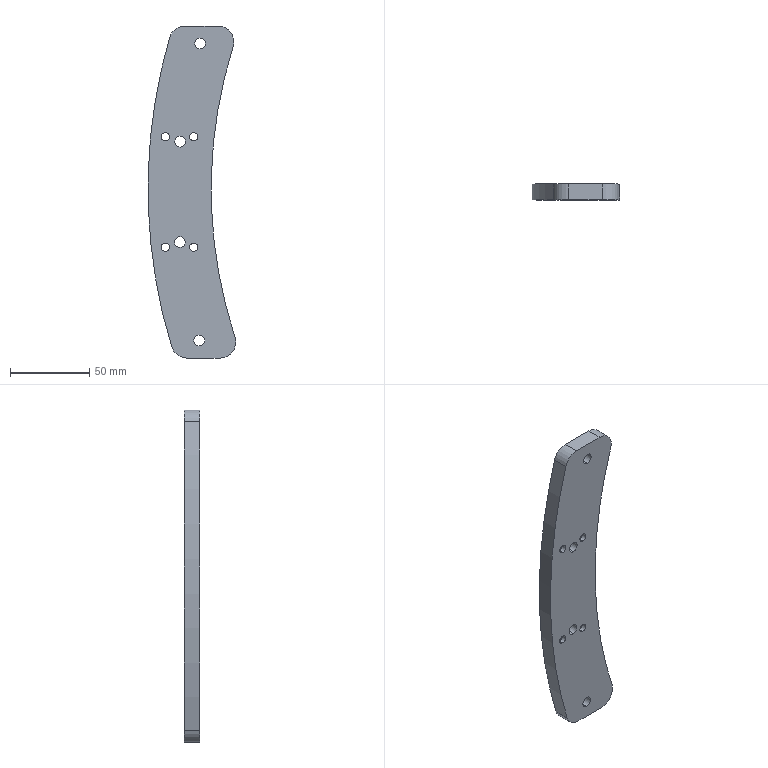Part | 1 solid | 38 faces | box 55.542 x 10 x 210 mm | volume 81183 mm3 | cylinder 30 | plane 8 | commonest cylinder face diameters 5.2 x8 6.8 x8 8.5 x8 20 x4 598 x1 682.4 x1
STEP:
#1=CARTESIAN_POINT('',(-4.991,3.,-65.75));
#2=VERTEX_POINT('',#1);
#3=CARTESIAN_POINT('',(-4.991,3.,-74.25));
#4=VERTEX_POINT('',#3);
#5=CARTESIAN_POINT('',(-4.991,3.,-70.));
#6=DIRECTION('',(0.,-1.,0.));
#7=DIRECTION('',(0.,0.,-1.));
#8=AXIS2_PLACEMENT_3D('',#5,#6,#7);
#9=CIRCLE('',#8,4.25);
#10=EDGE_CURVE('',#2,#4,#9,.T.);
#11=ORIENTED_EDGE('',*,*,#10,.T.);
#12=CARTESIAN_POINT('',(-4.991,10.,-74.25));
#13=VERTEX_POINT('',#12);
#14=CARTESIAN_POINT('',(-4.991,3.,-74.25));
#15=DIRECTION('',(0.,1.,0.));
#16=VECTOR('',#15,1000.);
#17=LINE('',#14,#16);
#18=EDGE_CURVE('',#4,#13,#17,.T.);
#19=ORIENTED_EDGE('',*,*,#18,.T.);
#20=CARTESIAN_POINT('',(-4.991,10.,-65.75));
#21=VERTEX_POINT('',#20);
#22=CARTESIAN_POINT('',(-4.991,10.,-70.));
#23=DIRECTION('',(0.,-1.,0.));
#24=DIRECTION('',(0.,0.,-1.));
#25=AXIS2_PLACEMENT_3D('',#22,#23,#24);
#26=CIRCLE('',#25,4.25);
#27=EDGE_CURVE('',#21,#13,#26,.T.);
#28=ORIENTED_EDGE('',*,*,#27,.F.);
#29=CARTESIAN_POINT('',(-4.991,3.,-65.75));
#30=DIRECTION('',(0.,1.,0.));
#31=VECTOR('',#30,1000.);
#32=LINE('',#29,#31);
#33=EDGE_CURVE('',#2,#21,#32,.T.);
#34=ORIENTED_EDGE('',*,*,#33,.F.);
#35=EDGE_LOOP('',(#11,#19,#28,#34));
#36=FACE_OUTER_BOUND('',#35,.T.);
#37=CARTESIAN_POINT('',(-4.991,3.,-70.));
#38=DIRECTION('',(0.,1.,0.));
#39=DIRECTION('',(0.,0.,1.));
#40=AXIS2_PLACEMENT_3D('',#37,#38,#39);
#41=CYLINDRICAL_SURFACE('',#40,4.25);
#42=ADVANCED_FACE('',(#36),#41,.F.);
#43=CARTESIAN_POINT('',(-4.991,3.,-135.75));
#44=VERTEX_POINT('',#43);
#45=CARTESIAN_POINT('',(-4.991,3.,-144.25));
#46=VERTEX_POINT('',#45);
#47=CARTESIAN_POINT('',(-4.991,3.,-140.));
#48=DIRECTION('',(0.,-1.,0.));
#49=DIRECTION('',(0.,0.,-1.));
#50=AXIS2_PLACEMENT_3D('',#47,#48,#49);
#51=CIRCLE('',#50,4.25);
#52=EDGE_CURVE('',#44,#46,#51,.T.);
#53=ORIENTED_EDGE('',*,*,#52,.T.);
#54=CARTESIAN_POINT('',(-4.991,10.,-144.25));
#55=VERTEX_POINT('',#54);
#56=CARTESIAN_POINT('',(-4.991,3.,-144.25));
#57=DIRECTION('',(0.,1.,0.));
#58=VECTOR('',#57,1000.);
#59=LINE('',#56,#58);
#60=EDGE_CURVE('',#46,#55,#59,.T.);
#61=ORIENTED_EDGE('',*,*,#60,.T.);
#62=CARTESIAN_POINT('',(-4.991,10.,-135.75));
#63=VERTEX_POINT('',#62);
#64=CARTESIAN_POINT('',(-4.991,10.,-140.));
#65=DIRECTION('',(0.,-1.,0.));
#66=DIRECTION('',(0.,0.,-1.));
#67=AXIS2_PLACEMENT_3D('',#64,#65,#66);
#68=CIRCLE('',#67,4.25);
#69=EDGE_CURVE('',#63,#55,#68,.T.);
#70=ORIENTED_EDGE('',*,*,#69,.F.);
#71=CARTESIAN_POINT('',(-4.991,3.,-135.75));
#72=DIRECTION('',(0.,1.,0.));
#73=VECTOR('',#72,1000.);
#74=LINE('',#71,#73);
#75=EDGE_CURVE('',#44,#63,#74,.T.);
#76=ORIENTED_EDGE('',*,*,#75,.F.);
#77=EDGE_LOOP('',(#53,#61,#70,#76));
#78=FACE_OUTER_BOUND('',#77,.T.);
#79=CARTESIAN_POINT('',(-4.991,3.,-140.));
#80=DIRECTION('',(0.,1.,0.));
#81=DIRECTION('',(0.,0.,1.));
#82=AXIS2_PLACEMENT_3D('',#79,#80,#81);
#83=CYLINDRICAL_SURFACE('',#82,4.25);
#84=ADVANCED_FACE('',(#78),#83,.F.);
#85=CARTESIAN_POINT('',(13.009,3.,-135.75));
#86=VERTEX_POINT('',#85);
#87=CARTESIAN_POINT('',(13.009,3.,-144.25));
#88=VERTEX_POINT('',#87);
#89=CARTESIAN_POINT('',(13.009,3.,-140.));
#90=DIRECTION('',(0.,-1.,0.));
#91=DIRECTION('',(0.,0.,-1.));
#92=AXIS2_PLACEMENT_3D('',#89,#90,#91);
#93=CIRCLE('',#92,4.25);
#94=EDGE_CURVE('',#86,#88,#93,.T.);
#95=ORIENTED_EDGE('',*,*,#94,.T.);
#96=CARTESIAN_POINT('',(13.009,10.,-144.25));
#97=VERTEX_POINT('',#96);
#98=CARTESIAN_POINT('',(13.009,3.,-144.25));
#99=DIRECTION('',(0.,1.,0.));
#100=VECTOR('',#99,1000.);
#101=LINE('',#98,#100);
#102=EDGE_CURVE('',#88,#97,#101,.T.);
#103=ORIENTED_EDGE('',*,*,#102,.T.);
#104=CARTESIAN_POINT('',(13.009,10.,-135.75));
#105=VERTEX_POINT('',#104);
#106=CARTESIAN_POINT('',(13.009,10.,-140.));
#107=DIRECTION('',(0.,-1.,0.));
#108=DIRECTION('',(0.,0.,-1.));
#109=AXIS2_PLACEMENT_3D('',#106,#107,#108);
#110=CIRCLE('',#109,4.25);
#111=EDGE_CURVE('',#105,#97,#110,.T.);
#112=ORIENTED_EDGE('',*,*,#111,.F.);
#113=CARTESIAN_POINT('',(13.009,3.,-135.75));
#114=DIRECTION('',(0.,1.,0.));
#115=VECTOR('',#114,1000.);
#116=LINE('',#113,#115);
#117=EDGE_CURVE('',#86,#105,#116,.T.);
#118=ORIENTED_EDGE('',*,*,#117,.F.);
#119=EDGE_LOOP('',(#95,#103,#112,#118));
#120=FACE_OUTER_BOUND('',#119,.T.);
#121=CARTESIAN_POINT('',(13.009,3.,-140.));
#122=DIRECTION('',(0.,1.,0.));
#123=DIRECTION('',(0.,0.,1.));
#124=AXIS2_PLACEMENT_3D('',#121,#122,#123);
#125=CYLINDRICAL_SURFACE('',#124,4.25);
#126=ADVANCED_FACE('',(#120),#125,.F.);
#127=CARTESIAN_POINT('',(13.009,3.,-65.75));
#128=VERTEX_POINT('',#127);
#129=CARTESIAN_POINT('',(13.009,3.,-74.25));
#130=VERTEX_POINT('',#129);
#131=CARTESIAN_POINT('',(13.009,3.,-70.));
#132=DIRECTION('',(0.,-1.,0.));
#133=DIRECTION('',(0.,0.,-1.));
#134=AXIS2_PLACEMENT_3D('',#131,#132,#133);
#135=CIRCLE('',#134,4.25);
#136=EDGE_CURVE('',#128,#130,#135,.T.);
#137=ORIENTED_EDGE('',*,*,#136,.T.);
#138=CARTESIAN_POINT('',(13.009,10.,-74.25));
#139=VERTEX_POINT('',#138);
#140=CARTESIAN_POINT('',(13.009,3.,-74.25));
#141=DIRECTION('',(0.,1.,0.));
#142=VECTOR('',#141,1000.);
#143=LINE('',#140,#142);
#144=EDGE_CURVE('',#130,#139,#143,.T.);
#145=ORIENTED_EDGE('',*,*,#144,.T.);
#146=CARTESIAN_POINT('',(13.009,10.,-65.75));
#147=VERTEX_POINT('',#146);
#148=CARTESIAN_POINT('',(13.009,10.,-70.));
#149=DIRECTION('',(0.,-1.,0.));
#150=DIRECTION('',(0.,0.,-1.));
#151=AXIS2_PLACEMENT_3D('',#148,#149,#150);
#152=CIRCLE('',#151,4.25);
#153=EDGE_CURVE('',#147,#139,#152,.T.);
#154=ORIENTED_EDGE('',*,*,#153,.F.);
#155=CARTESIAN_POINT('',(13.009,3.,-65.75));
#156=DIRECTION('',(0.,1.,0.));
#157=VECTOR('',#156,1000.);
#158=LINE('',#155,#157);
#159=EDGE_CURVE('',#128,#147,#158,.T.);
#160=ORIENTED_EDGE('',*,*,#159,.F.);
#161=EDGE_LOOP('',(#137,#145,#154,#160));
#162=FACE_OUTER_BOUND('',#161,.T.);
#163=CARTESIAN_POINT('',(13.009,3.,-70.));
#164=DIRECTION('',(0.,1.,0.));
#165=DIRECTION('',(0.,0.,1.));
#166=AXIS2_PLACEMENT_3D('',#163,#164,#165);
#167=CYLINDRICAL_SURFACE('',#166,4.25);
#168=ADVANCED_FACE('',(#162),#167,.F.);
#169=CARTESIAN_POINT('',(17.009,0.,-14.4));
#170=VERTEX_POINT('',#169);
#171=CARTESIAN_POINT('',(17.009,0.,-7.6));
#172=VERTEX_POINT('',#171);
#173=CARTESIAN_POINT('',(17.009,0.,-11.));
#174=DIRECTION('',(0.,1.,0.));
#175=DIRECTION('',(0.,0.,1.));
#176=AXIS2_PLACEMENT_3D('',#173,#174,#175);
#177=CIRCLE('',#176,3.4);
#178=EDGE_CURVE('',#170,#172,#177,.T.);
#179=ORIENTED_EDGE('',*,*,#178,.F.);
#180=CARTESIAN_POINT('',(17.009,10.,-14.4));
#181=VERTEX_POINT('',#180);
#182=CARTESIAN_POINT('',(17.009,10.,-14.4));
#183=DIRECTION('',(0.,1.,0.));
#184=VECTOR('',#183,1000.);
#185=LINE('',#182,#184);
#186=EDGE_CURVE('',#170,#181,#185,.T.);
#187=ORIENTED_EDGE('',*,*,#186,.T.);
#188=CARTESIAN_POINT('',(17.009,10.,-7.6));
#189=VERTEX_POINT('',#188);
#190=CARTESIAN_POINT('',(17.009,10.,-11.));
#191=DIRECTION('',(0.,1.,0.));
#192=DIRECTION('',(0.,0.,1.));
#193=AXIS2_PLACEMENT_3D('',#190,#191,#192);
#194=CIRCLE('',#193,3.4);
#195=EDGE_CURVE('',#181,#189,#194,.T.);
#196=ORIENTED_EDGE('',*,*,#195,.T.);
#197=CARTESIAN_POINT('',(17.009,10.,-7.6));
#198=DIRECTION('',(0.,1.,0.));
#199=VECTOR('',#198,1000.);
#200=LINE('',#197,#199);
#201=EDGE_CURVE('',#172,#189,#200,.T.);
#202=ORIENTED_EDGE('',*,*,#201,.F.);
#203=EDGE_LOOP('',(#179,#187,#196,#202));
#204=FACE_OUTER_BOUND('',#203,.T.);
#205=CARTESIAN_POINT('',(17.009,10.,-11.));
#206=DIRECTION('',(0.,1.,0.));
#207=DIRECTION('',(0.,0.,1.));
#208=AXIS2_PLACEMENT_3D('',#205,#206,#207);
#209=CYLINDRICAL_SURFACE('',#208,3.4);
#210=ADVANCED_FACE('',(#204),#209,.F.);
#211=CARTESIAN_POINT('',(16.509,0.,-202.4));
#212=VERTEX_POINT('',#211);
#213=CARTESIAN_POINT('',(16.509,0.,-195.6));
#214=VERTEX_POINT('',#213);
#215=CARTESIAN_POINT('',(16.509,0.,-199.));
#216=DIRECTION('',(0.,1.,0.));
#217=DIRECTION('',(0.,0.,1.));
#218=AXIS2_PLACEMENT_3D('',#215,#216,#217);
#219=CIRCLE('',#218,3.4);
#220=EDGE_CURVE('',#212,#214,#219,.T.);
#221=ORIENTED_EDGE('',*,*,#220,.F.);
#222=CARTESIAN_POINT('',(16.509,10.,-202.4));
#223=VERTEX_POINT('',#222);
#224=CARTESIAN_POINT('',(16.509,10.,-202.4));
#225=DIRECTION('',(0.,1.,0.));
#226=VECTOR('',#225,1000.);
#227=LINE('',#224,#226);
#228=EDGE_CURVE('',#212,#223,#227,.T.);
#229=ORIENTED_EDGE('',*,*,#228,.T.);
#230=CARTESIAN_POINT('',(16.509,10.,-195.6));
#231=VERTEX_POINT('',#230);
#232=CARTESIAN_POINT('',(16.509,10.,-199.));
#233=DIRECTION('',(0.,1.,0.));
#234=DIRECTION('',(0.,0.,1.));
#235=AXIS2_PLACEMENT_3D('',#232,#233,#234);
#236=CIRCLE('',#235,3.4);
#237=EDGE_CURVE('',#223,#231,#236,.T.);
#238=ORIENTED_EDGE('',*,*,#237,.T.);
#239=CARTESIAN_POINT('',(16.509,10.,-195.6));
#240=DIRECTION('',(0.,1.,0.));
#241=VECTOR('',#240,1000.);
#242=LINE('',#239,#241);
#243=EDGE_CURVE('',#214,#231,#242,.T.);
#244=ORIENTED_EDGE('',*,*,#243,.F.);
#245=EDGE_LOOP('',(#221,#229,#238,#244));
#246=FACE_OUTER_BOUND('',#245,.T.);
#247=CARTESIAN_POINT('',(16.509,10.,-199.));
#248=DIRECTION('',(0.,1.,0.));
#249=DIRECTION('',(0.,0.,1.));
#250=AXIS2_PLACEMENT_3D('',#247,#248,#249);
#251=CYLINDRICAL_SURFACE('',#250,3.4);
#252=ADVANCED_FACE('',(#246),#251,.F.);
#253=CARTESIAN_POINT('',(4.296,0.,-140.1));
#254=VERTEX_POINT('',#253);
#255=CARTESIAN_POINT('',(4.296,0.,-133.3));
#256=VERTEX_POINT('',#255);
#257=CARTESIAN_POINT('',(4.296,0.,-136.7));
#258=DIRECTION('',(0.,1.,0.));
#259=DIRECTION('',(0.,0.,1.));
#260=AXIS2_PLACEMENT_3D('',#257,#258,#259);
#261=CIRCLE('',#260,3.4);
#262=EDGE_CURVE('',#254,#256,#261,.T.);
#263=ORIENTED_EDGE('',*,*,#262,.F.);
#264=CARTESIAN_POINT('',(4.296,10.,-140.1));
#265=VERTEX_POINT('',#264);
#266=CARTESIAN_POINT('',(4.296,10.,-140.1));
#267=DIRECTION('',(0.,1.,0.));
#268=VECTOR('',#267,1000.);
#269=LINE('',#266,#268);
#270=EDGE_CURVE('',#254,#265,#269,.T.);
#271=ORIENTED_EDGE('',*,*,#270,.T.);
#272=CARTESIAN_POINT('',(4.296,10.,-133.3));
#273=VERTEX_POINT('',#272);
#274=CARTESIAN_POINT('',(4.296,10.,-136.7));
#275=DIRECTION('',(0.,1.,0.));
#276=DIRECTION('',(0.,0.,1.));
#277=AXIS2_PLACEMENT_3D('',#274,#275,#276);
#278=CIRCLE('',#277,3.4);
#279=EDGE_CURVE('',#265,#273,#278,.T.);
#280=ORIENTED_EDGE('',*,*,#279,.T.);
#281=CARTESIAN_POINT('',(4.296,10.,-133.3));
#282=DIRECTION('',(0.,1.,0.));
#283=VECTOR('',#282,1000.);
#284=LINE('',#281,#283);
#285=EDGE_CURVE('',#256,#273,#284,.T.);
#286=ORIENTED_EDGE('',*,*,#285,.F.);
#287=EDGE_LOOP('',(#263,#271,#280,#286));
#288=FACE_OUTER_BOUND('',#287,.T.);
#289=CARTESIAN_POINT('',(4.296,10.,-136.7));
#290=DIRECTION('',(0.,1.,0.));
#291=DIRECTION('',(0.,0.,1.));
#292=AXIS2_PLACEMENT_3D('',#289,#290,#291);
#293=CYLINDRICAL_SURFACE('',#292,3.4);
#294=ADVANCED_FACE('',(#288),#293,.F.);
#295=CARTESIAN_POINT('',(4.469,0.,-76.6));
#296=VERTEX_POINT('',#295);
#297=CARTESIAN_POINT('',(4.469,0.,-69.8));
#298=VERTEX_POINT('',#297);
#299=CARTESIAN_POINT('',(4.469,0.,-73.2));
#300=DIRECTION('',(0.,1.,0.));
#301=DIRECTION('',(0.,0.,1.));
#302=AXIS2_PLACEMENT_3D('',#299,#300,#301);
#303=CIRCLE('',#302,3.4);
#304=EDGE_CURVE('',#296,#298,#303,.T.);
#305=ORIENTED_EDGE('',*,*,#304,.F.);
#306=CARTESIAN_POINT('',(4.469,10.,-76.6));
#307=VERTEX_POINT('',#306);
#308=CARTESIAN_POINT('',(4.469,10.,-76.6));
#309=DIRECTION('',(0.,1.,0.));
#310=VECTOR('',#309,1000.);
#311=LINE('',#308,#310);
#312=EDGE_CURVE('',#296,#307,#311,.T.);
#313=ORIENTED_EDGE('',*,*,#312,.T.);
#314=CARTESIAN_POINT('',(4.469,10.,-69.8));
#315=VERTEX_POINT('',#314);
#316=CARTESIAN_POINT('',(4.469,10.,-73.2));
#317=DIRECTION('',(0.,1.,0.));
#318=DIRECTION('',(0.,0.,1.));
#319=AXIS2_PLACEMENT_3D('',#316,#317,#318);
#320=CIRCLE('',#319,3.4);
#321=EDGE_CURVE('',#307,#315,#320,.T.);
#322=ORIENTED_EDGE('',*,*,#321,.T.);
#323=CARTESIAN_POINT('',(4.469,10.,-69.8));
#324=DIRECTION('',(0.,1.,0.));
#325=VECTOR('',#324,1000.);
#326=LINE('',#323,#325);
#327=EDGE_CURVE('',#298,#315,#326,.T.);
#328=ORIENTED_EDGE('',*,*,#327,.F.);
#329=EDGE_LOOP('',(#305,#313,#322,#328));
#330=FACE_OUTER_BOUND('',#329,.T.);
#331=CARTESIAN_POINT('',(4.469,10.,-73.2));
#332=DIRECTION('',(0.,1.,0.));
#333=DIRECTION('',(0.,0.,1.));
#334=AXIS2_PLACEMENT_3D('',#331,#332,#333);
#335=CYLINDRICAL_SURFACE('',#334,3.4);
#336=ADVANCED_FACE('',(#330),#335,.F.);
#337=CARTESIAN_POINT('',(13.009,3.,-67.4));
#338=VERTEX_POINT('',#337);
#339=CARTESIAN_POINT('',(13.009,3.,-72.6));
#340=VERTEX_POINT('',#339);
#341=CARTESIAN_POINT('',(13.009,3.,-70.));
#342=DIRECTION('',(0.,-1.,0.));
#343=DIRECTION('',(0.,0.,-1.));
#344=AXIS2_PLACEMENT_3D('',#341,#342,#343);
#345=CIRCLE('',#344,2.6);
#346=EDGE_CURVE('',#338,#340,#345,.T.);
#347=ORIENTED_EDGE('',*,*,#346,.F.);
#348=CARTESIAN_POINT('',(13.009,0.,-67.4));
#349=VERTEX_POINT('',#348);
#350=CARTESIAN_POINT('',(13.009,10.,-67.4));
#351=DIRECTION('',(0.,-1.,0.));
#352=VECTOR('',#351,1000.);
#353=LINE('',#350,#352);
#354=EDGE_CURVE('',#338,#349,#353,.T.);
#355=ORIENTED_EDGE('',*,*,#354,.T.);
#356=CARTESIAN_POINT('',(13.009,0.,-72.6));
#357=VERTEX_POINT('',#356);
#358=CARTESIAN_POINT('',(13.009,0.,-70.));
#359=DIRECTION('',(0.,1.,0.));
#360=DIRECTION('',(0.,0.,1.));
#361=AXIS2_PLACEMENT_3D('',#358,#359,#360);
#362=CIRCLE('',#361,2.6);
#363=EDGE_CURVE('',#357,#349,#362,.T.);
#364=ORIENTED_EDGE('',*,*,#363,.F.);
#365=CARTESIAN_POINT('',(13.009,10.,-72.6));
#366=DIRECTION('',(0.,-1.,0.));
#367=VECTOR('',#366,1000.);
#368=LINE('',#365,#367);
#369=EDGE_CURVE('',#340,#357,#368,.T.);
#370=ORIENTED_EDGE('',*,*,#369,.F.);
#371=EDGE_LOOP('',(#347,#355,#364,#370));
#372=FACE_OUTER_BOUND('',#371,.T.);
#373=CARTESIAN_POINT('',(13.009,10.,-70.));
#374=DIRECTION('',(0.,-1.,0.));
#375=DIRECTION('',(0.,0.,-1.));
#376=AXIS2_PLACEMENT_3D('',#373,#374,#375);
#377=CYLINDRICAL_SURFACE('',#376,2.6);
#378=ADVANCED_FACE('',(#372),#377,.F.);
#379=CARTESIAN_POINT('',(13.009,3.,-137.4));
#380=VERTEX_POINT('',#379);
#381=CARTESIAN_POINT('',(13.009,3.,-142.6));
#382=VERTEX_POINT('',#381);
#383=CARTESIAN_POINT('',(13.009,3.,-140.));
#384=DIRECTION('',(0.,-1.,0.));
#385=DIRECTION('',(0.,0.,-1.));
#386=AXIS2_PLACEMENT_3D('',#383,#384,#385);
#387=CIRCLE('',#386,2.6);
#388=EDGE_CURVE('',#380,#382,#387,.T.);
#389=ORIENTED_EDGE('',*,*,#388,.F.);
#390=CARTESIAN_POINT('',(13.009,0.,-137.4));
#391=VERTEX_POINT('',#390);
#392=CARTESIAN_POINT('',(13.009,10.,-137.4));
#393=DIRECTION('',(0.,-1.,0.));
#394=VECTOR('',#393,1000.);
#395=LINE('',#392,#394);
#396=EDGE_CURVE('',#380,#391,#395,.T.);
#397=ORIENTED_EDGE('',*,*,#396,.T.);
#398=CARTESIAN_POINT('',(13.009,0.,-142.6));
#399=VERTEX_POINT('',#398);
#400=CARTESIAN_POINT('',(13.009,0.,-140.));
#401=DIRECTION('',(0.,1.,0.));
#402=DIRECTION('',(0.,0.,1.));
#403=AXIS2_PLACEMENT_3D('',#400,#401,#402);
#404=CIRCLE('',#403,2.6);
#405=EDGE_CURVE('',#399,#391,#404,.T.);
#406=ORIENTED_EDGE('',*,*,#405,.F.);
#407=CARTESIAN_POINT('',(13.009,10.,-142.6));
#408=DIRECTION('',(0.,-1.,0.));
#409=VECTOR('',#408,1000.);
#410=LINE('',#407,#409);
#411=EDGE_CURVE('',#382,#399,#410,.T.);
#412=ORIENTED_EDGE('',*,*,#411,.F.);
#413=EDGE_LOOP('',(#389,#397,#406,#412));
#414=FACE_OUTER_BOUND('',#413,.T.);
#415=CARTESIAN_POINT('',(13.009,10.,-140.));
#416=DIRECTION('',(0.,-1.,0.));
#417=DIRECTION('',(0.,0.,-1.));
#418=AXIS2_PLACEMENT_3D('',#415,#416,#417);
#419=CYLINDRICAL_SURFACE('',#418,2.6);
#420=ADVANCED_FACE('',(#414),#419,.F.);
#421=CARTESIAN_POINT('',(-4.991,3.,-137.4));
#422=VERTEX_POINT('',#421);
#423=CARTESIAN_POINT('',(-4.991,3.,-142.6));
#424=VERTEX_POINT('',#423);
#425=CARTESIAN_POINT('',(-4.991,3.,-140.));
#426=DIRECTION('',(0.,-1.,0.));
#427=DIRECTION('',(0.,0.,-1.));
#428=AXIS2_PLACEMENT_3D('',#425,#426,#427);
#429=CIRCLE('',#428,2.6);
#430=EDGE_CURVE('',#422,#424,#429,.T.);
#431=ORIENTED_EDGE('',*,*,#430,.F.);
#432=CARTESIAN_POINT('',(-4.991,0.,-137.4));
#433=VERTEX_POINT('',#432);
#434=CARTESIAN_POINT('',(-4.991,10.,-137.4));
#435=DIRECTION('',(0.,-1.,0.));
#436=VECTOR('',#435,1000.);
#437=LINE('',#434,#436);
#438=EDGE_CURVE('',#422,#433,#437,.T.);
#439=ORIENTED_EDGE('',*,*,#438,.T.);
#440=CARTESIAN_POINT('',(-4.991,0.,-142.6));
#441=VERTEX_POINT('',#440);
#442=CARTESIAN_POINT('',(-4.991,0.,-140.));
#443=DIRECTION('',(0.,1.,0.));
#444=DIRECTION('',(0.,0.,1.));
#445=AXIS2_PLACEMENT_3D('',#442,#443,#444);
#446=CIRCLE('',#445,2.6);
#447=EDGE_CURVE('',#441,#433,#446,.T.);
#448=ORIENTED_EDGE('',*,*,#447,.F.);
#449=CARTESIAN_POINT('',(-4.991,10.,-142.6));
#450=DIRECTION('',(0.,-1.,0.));
#451=VECTOR('',#450,1000.);
#452=LINE('',#449,#451);
#453=EDGE_CURVE('',#424,#441,#452,.T.);
#454=ORIENTED_EDGE('',*,*,#453,.F.);
#455=EDGE_LOOP('',(#431,#439,#448,#454));
#456=FACE_OUTER_BOUND('',#455,.T.);
#457=CARTESIAN_POINT('',(-4.991,10.,-140.));
#458=DIRECTION('',(0.,-1.,0.));
#459=DIRECTION('',(0.,0.,-1.));
#460=AXIS2_PLACEMENT_3D('',#457,#458,#459);
#461=CYLINDRICAL_SURFACE('',#460,2.6);
#462=ADVANCED_FACE('',(#456),#461,.F.);
#463=CARTESIAN_POINT('',(-4.991,3.,-67.4));
#464=VERTEX_POINT('',#463);
#465=CARTESIAN_POINT('',(-4.991,3.,-72.6));
#466=VERTEX_POINT('',#465);
#467=CARTESIAN_POINT('',(-4.991,3.,-70.));
#468=DIRECTION('',(0.,-1.,0.));
#469=DIRECTION('',(0.,0.,-1.));
#470=AXIS2_PLACEMENT_3D('',#467,#468,#469);
#471=CIRCLE('',#470,2.6);
#472=EDGE_CURVE('',#464,#466,#471,.T.);
#473=ORIENTED_EDGE('',*,*,#472,.F.);
#474=CARTESIAN_POINT('',(-4.991,0.,-67.4));
#475=VERTEX_POINT('',#474);
#476=CARTESIAN_POINT('',(-4.991,10.,-67.4));
#477=DIRECTION('',(0.,-1.,0.));
#478=VECTOR('',#477,1000.);
#479=LINE('',#476,#478);
#480=EDGE_CURVE('',#464,#475,#479,.T.);
#481=ORIENTED_EDGE('',*,*,#480,.T.);
#482=CARTESIAN_POINT('',(-4.991,0.,-72.6));
#483=VERTEX_POINT('',#482);
#484=CARTESIAN_POINT('',(-4.991,0.,-70.));
#485=DIRECTION('',(0.,1.,0.));
#486=DIRECTION('',(0.,0.,1.));
#487=AXIS2_PLACEMENT_3D('',#484,#485,#486);
#488=CIRCLE('',#487,2.6);
#489=EDGE_CURVE('',#483,#475,#488,.T.);
#490=ORIENTED_EDGE('',*,*,#489,.F.);
#491=CARTESIAN_POINT('',(-4.991,10.,-72.6));
#492=DIRECTION('',(0.,-1.,0.));
#493=VECTOR('',#492,1000.);
#494=LINE('',#491,#493);
#495=EDGE_CURVE('',#466,#483,#494,.T.);
#496=ORIENTED_EDGE('',*,*,#495,.F.);
#497=EDGE_LOOP('',(#473,#481,#490,#496));
#498=FACE_OUTER_BOUND('',#497,.T.);
#499=CARTESIAN_POINT('',(-4.991,10.,-70.));
#500=DIRECTION('',(0.,-1.,0.));
#501=DIRECTION('',(0.,0.,-1.));
#502=AXIS2_PLACEMENT_3D('',#499,#500,#501);
#503=CYLINDRICAL_SURFACE('',#502,2.6);
#504=ADVANCED_FACE('',(#498),#503,.F.);
#505=ORIENTED_EDGE('',*,*,#111,.T.);
#506=CARTESIAN_POINT('',(13.009,10.,-140.));
#507=DIRECTION('',(0.,-1.,0.));
#508=DIRECTION('',(0.,0.,-1.));
#509=AXIS2_PLACEMENT_3D('',#506,#507,#508);
#510=CIRCLE('',#509,4.25);
#511=EDGE_CURVE('',#97,#105,#510,.T.);
#512=ORIENTED_EDGE('',*,*,#511,.T.);
#513=EDGE_LOOP('',(#505,#512));
#514=FACE_BOUND('',#513,.T.);
#515=ORIENTED_EDGE('',*,*,#27,.T.);
#516=CARTESIAN_POINT('',(-4.991,10.,-70.));
#517=DIRECTION('',(0.,-1.,0.));
#518=DIRECTION('',(0.,0.,-1.));
#519=AXIS2_PLACEMENT_3D('',#516,#517,#518);
#520=CIRCLE('',#519,4.25);
#521=EDGE_CURVE('',#13,#21,#520,.T.);
#522=ORIENTED_EDGE('',*,*,#521,.T.);
#523=EDGE_LOOP('',(#515,#522));
#524=FACE_BOUND('',#523,.T.);
#525=ORIENTED_EDGE('',*,*,#153,.T.);
#526=CARTESIAN_POINT('',(13.009,10.,-70.));
#527=DIRECTION('',(0.,-1.,0.));
#528=DIRECTION('',(0.,0.,-1.));
#529=AXIS2_PLACEMENT_3D('',#526,#527,#528);
#530=CIRCLE('',#529,4.25);
#531=EDGE_CURVE('',#139,#147,#530,.T.);
#532=ORIENTED_EDGE('',*,*,#531,.T.);
#533=EDGE_LOOP('',(#525,#532));
#534=FACE_BOUND('',#533,.T.);
#535=ORIENTED_EDGE('',*,*,#69,.T.);
#536=CARTESIAN_POINT('',(-4.991,10.,-140.));
#537=DIRECTION('',(0.,-1.,0.));
#538=DIRECTION('',(0.,0.,-1.));
#539=AXIS2_PLACEMENT_3D('',#536,#537,#538);
#540=CIRCLE('',#539,4.25);
#541=EDGE_CURVE('',#55,#63,#540,.T.);
#542=ORIENTED_EDGE('',*,*,#541,.T.);
#543=EDGE_LOOP('',(#535,#542));
#544=FACE_BOUND('',#543,.T.);
#545=CARTESIAN_POINT('',(17.009,10.,-11.));
#546=DIRECTION('',(0.,1.,0.));
#547=DIRECTION('',(0.,0.,1.));
#548=AXIS2_PLACEMENT_3D('',#545,#546,#547);
#549=CIRCLE('',#548,3.4);
#550=EDGE_CURVE('',#189,#181,#549,.T.);
#551=ORIENTED_EDGE('',*,*,#550,.F.);
#552=ORIENTED_EDGE('',*,*,#195,.F.);
#553=EDGE_LOOP('',(#551,#552));
#554=FACE_BOUND('',#553,.T.);
#555=CARTESIAN_POINT('',(16.509,10.,-199.));
#556=DIRECTION('',(0.,1.,0.));
#557=DIRECTION('',(0.,0.,1.));
#558=AXIS2_PLACEMENT_3D('',#555,#556,#557);
#559=CIRCLE('',#558,3.4);
#560=EDGE_CURVE('',#231,#223,#559,.T.);
#561=ORIENTED_EDGE('',*,*,#560,.F.);
#562=ORIENTED_EDGE('',*,*,#237,.F.);
#563=EDGE_LOOP('',(#561,#562));
#564=FACE_BOUND('',#563,.T.);
#565=CARTESIAN_POINT('',(4.296,10.,-136.7));
#566=DIRECTION('',(0.,1.,0.));
#567=DIRECTION('',(0.,0.,1.));
#568=AXIS2_PLACEMENT_3D('',#565,#566,#567);
#569=CIRCLE('',#568,3.4);
#570=EDGE_CURVE('',#273,#265,#569,.T.);
#571=ORIENTED_EDGE('',*,*,#570,.F.);
#572=ORIENTED_EDGE('',*,*,#279,.F.);
#573=EDGE_LOOP('',(#571,#572));
#574=FACE_BOUND('',#573,.T.);
#575=CARTESIAN_POINT('',(4.469,10.,-73.2));
#576=DIRECTION('',(0.,1.,0.));
#577=DIRECTION('',(0.,0.,1.));
#578=AXIS2_PLACEMENT_3D('',#575,#576,#577);
#579=CIRCLE('',#578,3.4);
#580=EDGE_CURVE('',#315,#307,#579,.T.);
#581=ORIENTED_EDGE('',*,*,#580,.F.);
#582=ORIENTED_EDGE('',*,*,#321,.F.);
#583=EDGE_LOOP('',(#581,#582));
#584=FACE_BOUND('',#583,.T.);
#585=CARTESIAN_POINT('',(8.643,10.,-210.));
#586=VERTEX_POINT('',#585);
#587=CARTESIAN_POINT('',(-0.9179,10.,-202.931));
#588=VERTEX_POINT('',#587);
#589=CARTESIAN_POINT('',(8.643,10.,-200.));
#590=DIRECTION('',(0.,1.,0.));
#591=DIRECTION('',(0.,0.,1.));
#592=AXIS2_PLACEMENT_3D('',#589,#590,#591);
#593=CIRCLE('',#592,10.);
#594=EDGE_CURVE('',#586,#588,#593,.T.);
#595=ORIENTED_EDGE('',*,*,#594,.T.);
#596=CARTESIAN_POINT('',(-2.19,10.,-7.194));
#597=VERTEX_POINT('',#596);
#598=CARTESIAN_POINT('',(325.301,10.,-102.939));
#599=DIRECTION('',(0.,1.,0.));
#600=DIRECTION('',(0.,0.,1.));
#601=AXIS2_PLACEMENT_3D('',#598,#599,#600);
#602=CIRCLE('',#601,341.2);
#603=EDGE_CURVE('',#588,#597,#602,.T.);
#604=ORIENTED_EDGE('',*,*,#603,.T.);
#605=CARTESIAN_POINT('',(7.409,10.,0.));
#606=VERTEX_POINT('',#605);
#607=CARTESIAN_POINT('',(7.409,10.,-10.));
#608=DIRECTION('',(0.,1.,0.));
#609=DIRECTION('',(0.,0.,1.));
#610=AXIS2_PLACEMENT_3D('',#607,#608,#609);
#611=CIRCLE('',#610,10.);
#612=EDGE_CURVE('',#597,#606,#611,.T.);
#613=ORIENTED_EDGE('',*,*,#612,.T.);
#614=CARTESIAN_POINT('',(28.409,10.,0.));
#615=VERTEX_POINT('',#614);
#616=CARTESIAN_POINT('',(7.409,10.,0.));
#617=DIRECTION('',(1.,0.,0.));
#618=VECTOR('',#617,1000.);
#619=LINE('',#616,#618);
#620=EDGE_CURVE('',#606,#615,#619,.T.);
#621=ORIENTED_EDGE('',*,*,#620,.T.);
#622=CARTESIAN_POINT('',(37.944,10.,-13.013));
#623=VERTEX_POINT('',#622);
#624=CARTESIAN_POINT('',(28.409,10.,-10.));
#625=DIRECTION('',(0.,1.,0.));
#626=DIRECTION('',(0.,0.,-1.));
#627=AXIS2_PLACEMENT_3D('',#624,#625,#626);
#628=CIRCLE('',#627,10.);
#629=EDGE_CURVE('',#615,#623,#628,.T.);
#630=ORIENTED_EDGE('',*,*,#629,.T.);
#631=CARTESIAN_POINT('',(39.139,10.,-196.864));
#632=VERTEX_POINT('',#631);
#633=CARTESIAN_POINT('',(323.053,10.,-103.09));
#634=DIRECTION('',(0.,-1.,0.));
#635=DIRECTION('',(0.,0.,1.));
#636=AXIS2_PLACEMENT_3D('',#633,#634,#635);
#637=CIRCLE('',#636,299.);
#638=EDGE_CURVE('',#623,#632,#637,.T.);
#639=ORIENTED_EDGE('',*,*,#638,.T.);
#640=CARTESIAN_POINT('',(29.643,10.,-210.));
#641=VERTEX_POINT('',#640);
#642=CARTESIAN_POINT('',(29.643,10.,-200.));
#643=DIRECTION('',(0.,1.,0.));
#644=DIRECTION('',(0.,0.,-1.));
#645=AXIS2_PLACEMENT_3D('',#642,#643,#644);
#646=CIRCLE('',#645,10.);
#647=EDGE_CURVE('',#632,#641,#646,.T.);
#648=ORIENTED_EDGE('',*,*,#647,.T.);
#649=CARTESIAN_POINT('',(29.643,10.,-210.));
#650=DIRECTION('',(-1.,0.,0.));
#651=VECTOR('',#650,1000.);
#652=LINE('',#649,#651);
#653=EDGE_CURVE('',#641,#586,#652,.T.);
#654=ORIENTED_EDGE('',*,*,#653,.T.);
#655=EDGE_LOOP('',(#595,#604,#613,#621,#630,#639,#648,#654));
#656=FACE_OUTER_BOUND('',#655,.T.);
#657=CARTESIAN_POINT('',(8.643,10.,-200.));
#658=DIRECTION('',(0.,1.,0.));
#659=DIRECTION('',(0.,0.,1.));
#660=AXIS2_PLACEMENT_3D('',#657,#658,#659);
#661=PLANE('',#660);
#662=ADVANCED_FACE('',(#514,#524,#534,#544,#554,#564,#574,#584,#656),#661,.T.);
#663=CARTESIAN_POINT('',(17.009,0.,-11.));
#664=DIRECTION('',(0.,1.,0.));
#665=DIRECTION('',(0.,0.,1.));
#666=AXIS2_PLACEMENT_3D('',#663,#664,#665);
#667=CIRCLE('',#666,3.4);
#668=EDGE_CURVE('',#172,#170,#667,.T.);
#669=ORIENTED_EDGE('',*,*,#668,.T.);
#670=ORIENTED_EDGE('',*,*,#178,.T.);
#671=EDGE_LOOP('',(#669,#670));
#672=FACE_BOUND('',#671,.T.);
#673=CARTESIAN_POINT('',(16.509,0.,-199.));
#674=DIRECTION('',(0.,1.,0.));
#675=DIRECTION('',(0.,0.,1.));
#676=AXIS2_PLACEMENT_3D('',#673,#674,#675);
#677=CIRCLE('',#676,3.4);
#678=EDGE_CURVE('',#214,#212,#677,.T.);
#679=ORIENTED_EDGE('',*,*,#678,.T.);
#680=ORIENTED_EDGE('',*,*,#220,.T.);
#681=EDGE_LOOP('',(#679,#680));
#682=FACE_BOUND('',#681,.T.);
#683=CARTESIAN_POINT('',(4.296,0.,-136.7));
#684=DIRECTION('',(0.,1.,0.));
#685=DIRECTION('',(0.,0.,1.));
#686=AXIS2_PLACEMENT_3D('',#683,#684,#685);
#687=CIRCLE('',#686,3.4);
#688=EDGE_CURVE('',#256,#254,#687,.T.);
#689=ORIENTED_EDGE('',*,*,#688,.T.);
#690=ORIENTED_EDGE('',*,*,#262,.T.);
#691=EDGE_LOOP('',(#689,#690));
#692=FACE_BOUND('',#691,.T.);
#693=CARTESIAN_POINT('',(4.469,0.,-73.2));
#694=DIRECTION('',(0.,1.,0.));
#695=DIRECTION('',(0.,0.,1.));
#696=AXIS2_PLACEMENT_3D('',#693,#694,#695);
#697=CIRCLE('',#696,3.4);
#698=EDGE_CURVE('',#298,#296,#697,.T.);
#699=ORIENTED_EDGE('',*,*,#698,.T.);
#700=ORIENTED_EDGE('',*,*,#304,.T.);
#701=EDGE_LOOP('',(#699,#700));
#702=FACE_BOUND('',#701,.T.);
#703=CARTESIAN_POINT('',(8.643,0.,-210.));
#704=VERTEX_POINT('',#703);
#705=CARTESIAN_POINT('',(-0.9179,0.,-202.931));
#706=VERTEX_POINT('',#705);
#707=CARTESIAN_POINT('',(8.643,0.,-200.));
#708=DIRECTION('',(0.,1.,0.));
#709=DIRECTION('',(0.,0.,1.));
#710=AXIS2_PLACEMENT_3D('',#707,#708,#709);
#711=CIRCLE('',#710,10.);
#712=EDGE_CURVE('',#704,#706,#711,.T.);
#713=ORIENTED_EDGE('',*,*,#712,.F.);
#714=CARTESIAN_POINT('',(29.643,0.,-210.));
#715=VERTEX_POINT('',#714);
#716=CARTESIAN_POINT('',(29.643,0.,-210.));
#717=DIRECTION('',(-1.,0.,0.));
#718=VECTOR('',#717,1000.);
#719=LINE('',#716,#718);
#720=EDGE_CURVE('',#715,#704,#719,.T.);
#721=ORIENTED_EDGE('',*,*,#720,.F.);
#722=CARTESIAN_POINT('',(39.139,0.,-196.864));
#723=VERTEX_POINT('',#722);
#724=CARTESIAN_POINT('',(29.643,0.,-200.));
#725=DIRECTION('',(0.,1.,0.));
#726=DIRECTION('',(0.,0.,-1.));
#727=AXIS2_PLACEMENT_3D('',#724,#725,#726);
#728=CIRCLE('',#727,10.);
#729=EDGE_CURVE('',#723,#715,#728,.T.);
#730=ORIENTED_EDGE('',*,*,#729,.F.);
#731=CARTESIAN_POINT('',(37.944,0.,-13.013));
#732=VERTEX_POINT('',#731);
#733=CARTESIAN_POINT('',(323.053,0.,-103.09));
#734=DIRECTION('',(0.,-1.,0.));
#735=DIRECTION('',(0.,0.,1.));
#736=AXIS2_PLACEMENT_3D('',#733,#734,#735);
#737=CIRCLE('',#736,299.);
#738=EDGE_CURVE('',#732,#723,#737,.T.);
#739=ORIENTED_EDGE('',*,*,#738,.F.);
#740=CARTESIAN_POINT('',(28.409,0.,0.));
#741=VERTEX_POINT('',#740);
#742=CARTESIAN_POINT('',(28.409,0.,-10.));
#743=DIRECTION('',(0.,1.,0.));
#744=DIRECTION('',(0.,0.,-1.));
#745=AXIS2_PLACEMENT_3D('',#742,#743,#744);
#746=CIRCLE('',#745,10.);
#747=EDGE_CURVE('',#741,#732,#746,.T.);
#748=ORIENTED_EDGE('',*,*,#747,.F.);
#749=CARTESIAN_POINT('',(7.409,0.,0.));
#750=VERTEX_POINT('',#749);
#751=CARTESIAN_POINT('',(7.409,0.,0.));
#752=DIRECTION('',(1.,0.,0.));
#753=VECTOR('',#752,1000.);
#754=LINE('',#751,#753);
#755=EDGE_CURVE('',#750,#741,#754,.T.);
#756=ORIENTED_EDGE('',*,*,#755,.F.);
#757=CARTESIAN_POINT('',(-2.19,0.,-7.194));
#758=VERTEX_POINT('',#757);
#759=CARTESIAN_POINT('',(7.409,0.,-10.));
#760=DIRECTION('',(0.,1.,0.));
#761=DIRECTION('',(0.,0.,1.));
#762=AXIS2_PLACEMENT_3D('',#759,#760,#761);
#763=CIRCLE('',#762,10.);
#764=EDGE_CURVE('',#758,#750,#763,.T.);
#765=ORIENTED_EDGE('',*,*,#764,.F.);
#766=CARTESIAN_POINT('',(325.301,0.,-102.939));
#767=DIRECTION('',(0.,1.,0.));
#768=DIRECTION('',(0.,0.,1.));
#769=AXIS2_PLACEMENT_3D('',#766,#767,#768);
#770=CIRCLE('',#769,341.2);
#771=EDGE_CURVE('',#706,#758,#770,.T.);
#772=ORIENTED_EDGE('',*,*,#771,.F.);
#773=EDGE_LOOP('',(#713,#721,#730,#739,#748,#756,#765,#772));
#774=FACE_OUTER_BOUND('',#773,.T.);
#775=ORIENTED_EDGE('',*,*,#489,.T.);
#776=CARTESIAN_POINT('',(-4.991,0.,-70.));
#777=DIRECTION('',(0.,1.,0.));
#778=DIRECTION('',(0.,0.,1.));
#779=AXIS2_PLACEMENT_3D('',#776,#777,#778);
#780=CIRCLE('',#779,2.6);
#781=EDGE_CURVE('',#475,#483,#780,.T.);
#782=ORIENTED_EDGE('',*,*,#781,.T.);
#783=EDGE_LOOP('',(#775,#782));
#784=FACE_BOUND('',#783,.T.);
#785=ORIENTED_EDGE('',*,*,#447,.T.);
#786=CARTESIAN_POINT('',(-4.991,0.,-140.));
#787=DIRECTION('',(0.,1.,0.));
#788=DIRECTION('',(0.,0.,1.));
#789=AXIS2_PLACEMENT_3D('',#786,#787,#788);
#790=CIRCLE('',#789,2.6);
#791=EDGE_CURVE('',#433,#441,#790,.T.);
#792=ORIENTED_EDGE('',*,*,#791,.T.);
#793=EDGE_LOOP('',(#785,#792));
#794=FACE_BOUND('',#793,.T.);
#795=ORIENTED_EDGE('',*,*,#405,.T.);
#796=CARTESIAN_POINT('',(13.009,0.,-140.));
#797=DIRECTION('',(0.,1.,0.));
#798=DIRECTION('',(0.,0.,1.));
#799=AXIS2_PLACEMENT_3D('',#796,#797,#798);
#800=CIRCLE('',#799,2.6);
#801=EDGE_CURVE('',#391,#399,#800,.T.);
#802=ORIENTED_EDGE('',*,*,#801,.T.);
#803=EDGE_LOOP('',(#795,#802));
#804=FACE_BOUND('',#803,.T.);
#805=ORIENTED_EDGE('',*,*,#363,.T.);
#806=CARTESIAN_POINT('',(13.009,0.,-70.));
#807=DIRECTION('',(0.,1.,0.));
#808=DIRECTION('',(0.,0.,1.));
#809=AXIS2_PLACEMENT_3D('',#806,#807,#808);
#810=CIRCLE('',#809,2.6);
#811=EDGE_CURVE('',#349,#357,#810,.T.);
#812=ORIENTED_EDGE('',*,*,#811,.T.);
#813=EDGE_LOOP('',(#805,#812));
#814=FACE_BOUND('',#813,.T.);
#815=CARTESIAN_POINT('',(8.643,0.,-200.));
#816=DIRECTION('',(0.,1.,0.));
#817=DIRECTION('',(0.,0.,1.));
#818=AXIS2_PLACEMENT_3D('',#815,#816,#817);
#819=PLANE('',#818);
#820=ADVANCED_FACE('',(#672,#682,#692,#702,#774,#784,#794,#804,#814),#819,.F.);
#821=ORIENTED_EDGE('',*,*,#712,.T.);
#822=CARTESIAN_POINT('',(-0.9179,10.,-202.931));
#823=DIRECTION('',(0.,-1.,0.));
#824=VECTOR('',#823,1000.);
#825=LINE('',#822,#824);
#826=EDGE_CURVE('',#588,#706,#825,.T.);
#827=ORIENTED_EDGE('',*,*,#826,.F.);
#828=ORIENTED_EDGE('',*,*,#594,.F.);
#829=CARTESIAN_POINT('',(8.643,10.,-210.));
#830=DIRECTION('',(0.,-1.,0.));
#831=VECTOR('',#830,1000.);
#832=LINE('',#829,#831);
#833=EDGE_CURVE('',#586,#704,#832,.T.);
#834=ORIENTED_EDGE('',*,*,#833,.T.);
#835=EDGE_LOOP('',(#821,#827,#828,#834));
#836=FACE_OUTER_BOUND('',#835,.T.);
#837=CARTESIAN_POINT('',(8.643,10.,-200.));
#838=DIRECTION('',(0.,-1.,0.));
#839=DIRECTION('',(0.,0.,-1.));
#840=AXIS2_PLACEMENT_3D('',#837,#838,#839);
#841=CYLINDRICAL_SURFACE('',#840,10.);
#842=ADVANCED_FACE('',(#836),#841,.T.);
#843=ORIENTED_EDGE('',*,*,#771,.T.);
#844=CARTESIAN_POINT('',(-2.19,10.,-7.194));
#845=DIRECTION('',(0.,-1.,0.));
#846=VECTOR('',#845,1000.);
#847=LINE('',#844,#846);
#848=EDGE_CURVE('',#597,#758,#847,.T.);
#849=ORIENTED_EDGE('',*,*,#848,.F.);
#850=ORIENTED_EDGE('',*,*,#603,.F.);
#851=ORIENTED_EDGE('',*,*,#826,.T.);
#852=EDGE_LOOP('',(#843,#849,#850,#851));
#853=FACE_OUTER_BOUND('',#852,.T.);
#854=CARTESIAN_POINT('',(325.301,10.,-102.939));
#855=DIRECTION('',(0.,-1.,0.));
#856=DIRECTION('',(0.,0.,-1.));
#857=AXIS2_PLACEMENT_3D('',#854,#855,#856);
#858=CYLINDRICAL_SURFACE('',#857,341.2);
#859=ADVANCED_FACE('',(#853),#858,.T.);
#860=ORIENTED_EDGE('',*,*,#764,.T.);
#861=CARTESIAN_POINT('',(7.409,10.,0.));
#862=DIRECTION('',(0.,-1.,0.));
#863=VECTOR('',#862,1000.);
#864=LINE('',#861,#863);
#865=EDGE_CURVE('',#606,#750,#864,.T.);
#866=ORIENTED_EDGE('',*,*,#865,.F.);
#867=ORIENTED_EDGE('',*,*,#612,.F.);
#868=ORIENTED_EDGE('',*,*,#848,.T.);
#869=EDGE_LOOP('',(#860,#866,#867,#868));
#870=FACE_OUTER_BOUND('',#869,.T.);
#871=CARTESIAN_POINT('',(7.409,10.,-10.));
#872=DIRECTION('',(0.,-1.,0.));
#873=DIRECTION('',(0.,0.,-1.));
#874=AXIS2_PLACEMENT_3D('',#871,#872,#873);
#875=CYLINDRICAL_SURFACE('',#874,10.);
#876=ADVANCED_FACE('',(#870),#875,.T.);
#877=ORIENTED_EDGE('',*,*,#755,.T.);
#878=CARTESIAN_POINT('',(28.409,10.,0.));
#879=DIRECTION('',(0.,-1.,0.));
#880=VECTOR('',#879,1000.);
#881=LINE('',#878,#880);
#882=EDGE_CURVE('',#615,#741,#881,.T.);
#883=ORIENTED_EDGE('',*,*,#882,.F.);
#884=ORIENTED_EDGE('',*,*,#620,.F.);
#885=ORIENTED_EDGE('',*,*,#865,.T.);
#886=EDGE_LOOP('',(#877,#883,#884,#885));
#887=FACE_OUTER_BOUND('',#886,.T.);
#888=CARTESIAN_POINT('',(7.409,10.,0.));
#889=DIRECTION('',(0.,0.,-1.));
#890=DIRECTION('',(-1.,0.,0.));
#891=AXIS2_PLACEMENT_3D('',#888,#889,#890);
#892=PLANE('',#891);
#893=ADVANCED_FACE('',(#887),#892,.F.);
#894=ORIENTED_EDGE('',*,*,#747,.T.);
#895=CARTESIAN_POINT('',(37.944,10.,-13.013));
#896=DIRECTION('',(0.,-1.,0.));
#897=VECTOR('',#896,1000.);
#898=LINE('',#895,#897);
#899=EDGE_CURVE('',#623,#732,#898,.T.);
#900=ORIENTED_EDGE('',*,*,#899,.F.);
#901=ORIENTED_EDGE('',*,*,#629,.F.);
#902=ORIENTED_EDGE('',*,*,#882,.T.);
#903=EDGE_LOOP('',(#894,#900,#901,#902));
#904=FACE_OUTER_BOUND('',#903,.T.);
#905=CARTESIAN_POINT('',(28.409,10.,-10.));
#906=DIRECTION('',(0.,-1.,0.));
#907=DIRECTION('',(0.,0.,-1.));
#908=AXIS2_PLACEMENT_3D('',#905,#906,#907);
#909=CYLINDRICAL_SURFACE('',#908,10.);
#910=ADVANCED_FACE('',(#904),#909,.T.);
#911=ORIENTED_EDGE('',*,*,#738,.T.);
#912=CARTESIAN_POINT('',(39.139,10.,-196.864));
#913=DIRECTION('',(0.,-1.,0.));
#914=VECTOR('',#913,1000.);
#915=LINE('',#912,#914);
#916=EDGE_CURVE('',#632,#723,#915,.T.);
#917=ORIENTED_EDGE('',*,*,#916,.F.);
#918=ORIENTED_EDGE('',*,*,#638,.F.);
#919=ORIENTED_EDGE('',*,*,#899,.T.);
#920=EDGE_LOOP('',(#911,#917,#918,#919));
#921=FACE_OUTER_BOUND('',#920,.T.);
#922=CARTESIAN_POINT('',(323.053,10.,-103.09));
#923=DIRECTION('',(0.,-1.,0.));
#924=DIRECTION('',(0.,0.,-1.));
#925=AXIS2_PLACEMENT_3D('',#922,#923,#924);
#926=CYLINDRICAL_SURFACE('',#925,299.);
#927=ADVANCED_FACE('',(#921),#926,.F.);
#928=ORIENTED_EDGE('',*,*,#729,.T.);
#929=CARTESIAN_POINT('',(29.643,10.,-210.));
#930=DIRECTION('',(0.,-1.,0.));
#931=VECTOR('',#930,1000.);
#932=LINE('',#929,#931);
#933=EDGE_CURVE('',#641,#715,#932,.T.);
#934=ORIENTED_EDGE('',*,*,#933,.F.);
#935=ORIENTED_EDGE('',*,*,#647,.F.);
#936=ORIENTED_EDGE('',*,*,#916,.T.);
#937=EDGE_LOOP('',(#928,#934,#935,#936));
#938=FACE_OUTER_BOUND('',#937,.T.);
#939=CARTESIAN_POINT('',(29.643,10.,-200.));
#940=DIRECTION('',(0.,-1.,0.));
#941=DIRECTION('',(0.,0.,-1.));
#942=AXIS2_PLACEMENT_3D('',#939,#940,#941);
#943=CYLINDRICAL_SURFACE('',#942,10.);
#944=ADVANCED_FACE('',(#938),#943,.T.);
#945=ORIENTED_EDGE('',*,*,#720,.T.);
#946=ORIENTED_EDGE('',*,*,#833,.F.);
#947=ORIENTED_EDGE('',*,*,#653,.F.);
#948=ORIENTED_EDGE('',*,*,#933,.T.);
#949=EDGE_LOOP('',(#945,#946,#947,#948));
#950=FACE_OUTER_BOUND('',#949,.T.);
#951=CARTESIAN_POINT('',(29.643,10.,-210.));
#952=DIRECTION('',(0.,0.,1.));
#953=DIRECTION('',(1.,0.,0.));
#954=AXIS2_PLACEMENT_3D('',#951,#952,#953);
#955=PLANE('',#954);
#956=ADVANCED_FACE('',(#950),#955,.F.);
#957=ORIENTED_EDGE('',*,*,#480,.F.);
#958=CARTESIAN_POINT('',(-4.991,3.,-70.));
#959=DIRECTION('',(0.,-1.,0.));
#960=DIRECTION('',(0.,0.,-1.));
#961=AXIS2_PLACEMENT_3D('',#958,#959,#960);
#962=CIRCLE('',#961,2.6);
#963=EDGE_CURVE('',#466,#464,#962,.T.);
#964=ORIENTED_EDGE('',*,*,#963,.F.);
#965=ORIENTED_EDGE('',*,*,#495,.T.);
#966=ORIENTED_EDGE('',*,*,#781,.F.);
#967=EDGE_LOOP('',(#957,#964,#965,#966));
#968=FACE_OUTER_BOUND('',#967,.T.);
#969=CARTESIAN_POINT('',(-4.991,10.,-70.));
#970=DIRECTION('',(0.,-1.,0.));
#971=DIRECTION('',(0.,0.,-1.));
#972=AXIS2_PLACEMENT_3D('',#969,#970,#971);
#973=CYLINDRICAL_SURFACE('',#972,2.6);
#974=ADVANCED_FACE('',(#968),#973,.F.);
#975=ORIENTED_EDGE('',*,*,#438,.F.);
#976=CARTESIAN_POINT('',(-4.991,3.,-140.));
#977=DIRECTION('',(0.,-1.,0.));
#978=DIRECTION('',(0.,0.,-1.));
#979=AXIS2_PLACEMENT_3D('',#976,#977,#978);
#980=CIRCLE('',#979,2.6);
#981=EDGE_CURVE('',#424,#422,#980,.T.);
#982=ORIENTED_EDGE('',*,*,#981,.F.);
#983=ORIENTED_EDGE('',*,*,#453,.T.);
#984=ORIENTED_EDGE('',*,*,#791,.F.);
#985=EDGE_LOOP('',(#975,#982,#983,#984));
#986=FACE_OUTER_BOUND('',#985,.T.);
#987=CARTESIAN_POINT('',(-4.991,10.,-140.));
#988=DIRECTION('',(0.,-1.,0.));
#989=DIRECTION('',(0.,0.,-1.));
#990=AXIS2_PLACEMENT_3D('',#987,#988,#989);
#991=CYLINDRICAL_SURFACE('',#990,2.6);
#992=ADVANCED_FACE('',(#986),#991,.F.);
#993=ORIENTED_EDGE('',*,*,#396,.F.);
#994=CARTESIAN_POINT('',(13.009,3.,-140.));
#995=DIRECTION('',(0.,-1.,0.));
#996=DIRECTION('',(0.,0.,-1.));
#997=AXIS2_PLACEMENT_3D('',#994,#995,#996);
#998=CIRCLE('',#997,2.6);
#999=EDGE_CURVE('',#382,#380,#998,.T.);
#1000=ORIENTED_EDGE('',*,*,#999,.F.);
#1001=ORIENTED_EDGE('',*,*,#411,.T.);
#1002=ORIENTED_EDGE('',*,*,#801,.F.);
#1003=EDGE_LOOP('',(#993,#1000,#1001,#1002));
#1004=FACE_OUTER_BOUND('',#1003,.T.);
#1005=CARTESIAN_POINT('',(13.009,10.,-140.));
#1006=DIRECTION('',(0.,-1.,0.));
#1007=DIRECTION('',(0.,0.,-1.));
#1008=AXIS2_PLACEMENT_3D('',#1005,#1006,#1007);
#1009=CYLINDRICAL_SURFACE('',#1008,2.6);
#1010=ADVANCED_FACE('',(#1004),#1009,.F.);
#1011=ORIENTED_EDGE('',*,*,#354,.F.);
#1012=CARTESIAN_POINT('',(13.009,3.,-70.));
#1013=DIRECTION('',(0.,-1.,0.));
#1014=DIRECTION('',(0.,0.,-1.));
#1015=AXIS2_PLACEMENT_3D('',#1012,#1013,#1014);
#1016=CIRCLE('',#1015,2.6);
#1017=EDGE_CURVE('',#340,#338,#1016,.T.);
#1018=ORIENTED_EDGE('',*,*,#1017,.F.);
#1019=ORIENTED_EDGE('',*,*,#369,.T.);
#1020=ORIENTED_EDGE('',*,*,#811,.F.);
#1021=EDGE_LOOP('',(#1011,#1018,#1019,#1020));
#1022=FACE_OUTER_BOUND('',#1021,.T.);
#1023=CARTESIAN_POINT('',(13.009,10.,-70.));
#1024=DIRECTION('',(0.,-1.,0.));
#1025=DIRECTION('',(0.,0.,-1.));
#1026=AXIS2_PLACEMENT_3D('',#1023,#1024,#1025);
#1027=CYLINDRICAL_SURFACE('',#1026,2.6);
#1028=ADVANCED_FACE('',(#1022),#1027,.F.);
#1029=ORIENTED_EDGE('',*,*,#312,.F.);
#1030=ORIENTED_EDGE('',*,*,#698,.F.);
#1031=ORIENTED_EDGE('',*,*,#327,.T.);
#1032=ORIENTED_EDGE('',*,*,#580,.T.);
#1033=EDGE_LOOP('',(#1029,#1030,#1031,#1032));
#1034=FACE_OUTER_BOUND('',#1033,.T.);
#1035=CARTESIAN_POINT('',(4.469,10.,-73.2));
#1036=DIRECTION('',(0.,1.,0.));
#1037=DIRECTION('',(0.,0.,1.));
#1038=AXIS2_PLACEMENT_3D('',#1035,#1036,#1037);
#1039=CYLINDRICAL_SURFACE('',#1038,3.4);
#1040=ADVANCED_FACE('',(#1034),#1039,.F.);
#1041=ORIENTED_EDGE('',*,*,#270,.F.);
#1042=ORIENTED_EDGE('',*,*,#688,.F.);
#1043=ORIENTED_EDGE('',*,*,#285,.T.);
#1044=ORIENTED_EDGE('',*,*,#570,.T.);
#1045=EDGE_LOOP('',(#1041,#1042,#1043,#1044));
#1046=FACE_OUTER_BOUND('',#1045,.T.);
#1047=CARTESIAN_POINT('',(4.296,10.,-136.7));
#1048=DIRECTION('',(0.,1.,0.));
#1049=DIRECTION('',(0.,0.,1.));
#1050=AXIS2_PLACEMENT_3D('',#1047,#1048,#1049);
#1051=CYLINDRICAL_SURFACE('',#1050,3.4);
#1052=ADVANCED_FACE('',(#1046),#1051,.F.);
#1053=ORIENTED_EDGE('',*,*,#228,.F.);
#1054=ORIENTED_EDGE('',*,*,#678,.F.);
#1055=ORIENTED_EDGE('',*,*,#243,.T.);
#1056=ORIENTED_EDGE('',*,*,#560,.T.);
#1057=EDGE_LOOP('',(#1053,#1054,#1055,#1056));
#1058=FACE_OUTER_BOUND('',#1057,.T.);
#1059=CARTESIAN_POINT('',(16.509,10.,-199.));
#1060=DIRECTION('',(0.,1.,0.));
#1061=DIRECTION('',(0.,0.,1.));
#1062=AXIS2_PLACEMENT_3D('',#1059,#1060,#1061);
#1063=CYLINDRICAL_SURFACE('',#1062,3.4);
#1064=ADVANCED_FACE('',(#1058),#1063,.F.);
#1065=ORIENTED_EDGE('',*,*,#186,.F.);
#1066=ORIENTED_EDGE('',*,*,#668,.F.);
#1067=ORIENTED_EDGE('',*,*,#201,.T.);
#1068=ORIENTED_EDGE('',*,*,#550,.T.);
#1069=EDGE_LOOP('',(#1065,#1066,#1067,#1068));
#1070=FACE_OUTER_BOUND('',#1069,.T.);
#1071=CARTESIAN_POINT('',(17.009,10.,-11.));
#1072=DIRECTION('',(0.,1.,0.));
#1073=DIRECTION('',(0.,0.,1.));
#1074=AXIS2_PLACEMENT_3D('',#1071,#1072,#1073);
#1075=CYLINDRICAL_SURFACE('',#1074,3.4);
#1076=ADVANCED_FACE('',(#1070),#1075,.F.);
#1077=ORIENTED_EDGE('',*,*,#144,.F.);
#1078=CARTESIAN_POINT('',(13.009,3.,-70.));
#1079=DIRECTION('',(0.,-1.,0.));
#1080=DIRECTION('',(0.,0.,-1.));
#1081=AXIS2_PLACEMENT_3D('',#1078,#1079,#1080);
#1082=CIRCLE('',#1081,4.25);
#1083=EDGE_CURVE('',#130,#128,#1082,.T.);
#1084=ORIENTED_EDGE('',*,*,#1083,.T.);
#1085=ORIENTED_EDGE('',*,*,#159,.T.);
#1086=ORIENTED_EDGE('',*,*,#531,.F.);
#1087=EDGE_LOOP('',(#1077,#1084,#1085,#1086));
#1088=FACE_OUTER_BOUND('',#1087,.T.);
#1089=CARTESIAN_POINT('',(13.009,3.,-70.));
#1090=DIRECTION('',(0.,1.,0.));
#1091=DIRECTION('',(0.,0.,1.));
#1092=AXIS2_PLACEMENT_3D('',#1089,#1090,#1091);
#1093=CYLINDRICAL_SURFACE('',#1092,4.25);
#1094=ADVANCED_FACE('',(#1088),#1093,.F.);
#1095=ORIENTED_EDGE('',*,*,#1017,.T.);
#1096=ORIENTED_EDGE('',*,*,#346,.T.);
#1097=EDGE_LOOP('',(#1095,#1096));
#1098=FACE_BOUND('',#1097,.T.);
#1099=ORIENTED_EDGE('',*,*,#136,.F.);
#1100=ORIENTED_EDGE('',*,*,#1083,.F.);
#1101=EDGE_LOOP('',(#1099,#1100));
#1102=FACE_OUTER_BOUND('',#1101,.T.);
#1103=CARTESIAN_POINT('',(13.009,3.,-70.));
#1104=DIRECTION('',(0.,-1.,0.));
#1105=DIRECTION('',(0.,0.,-1.));
#1106=AXIS2_PLACEMENT_3D('',#1103,#1104,#1105);
#1107=PLANE('',#1106);
#1108=ADVANCED_FACE('',(#1098,#1102),#1107,.F.);
#1109=ORIENTED_EDGE('',*,*,#102,.F.);
#1110=CARTESIAN_POINT('',(13.009,3.,-140.));
#1111=DIRECTION('',(0.,-1.,0.));
#1112=DIRECTION('',(0.,0.,-1.));
#1113=AXIS2_PLACEMENT_3D('',#1110,#1111,#1112);
#1114=CIRCLE('',#1113,4.25);
#1115=EDGE_CURVE('',#88,#86,#1114,.T.);
#1116=ORIENTED_EDGE('',*,*,#1115,.T.);
#1117=ORIENTED_EDGE('',*,*,#117,.T.);
#1118=ORIENTED_EDGE('',*,*,#511,.F.);
#1119=EDGE_LOOP('',(#1109,#1116,#1117,#1118));
#1120=FACE_OUTER_BOUND('',#1119,.T.);
#1121=CARTESIAN_POINT('',(13.009,3.,-140.));
#1122=DIRECTION('',(0.,1.,0.));
#1123=DIRECTION('',(0.,0.,1.));
#1124=AXIS2_PLACEMENT_3D('',#1121,#1122,#1123);
#1125=CYLINDRICAL_SURFACE('',#1124,4.25);
#1126=ADVANCED_FACE('',(#1120),#1125,.F.);
#1127=ORIENTED_EDGE('',*,*,#999,.T.);
#1128=ORIENTED_EDGE('',*,*,#388,.T.);
#1129=EDGE_LOOP('',(#1127,#1128));
#1130=FACE_BOUND('',#1129,.T.);
#1131=ORIENTED_EDGE('',*,*,#94,.F.);
#1132=ORIENTED_EDGE('',*,*,#1115,.F.);
#1133=EDGE_LOOP('',(#1131,#1132));
#1134=FACE_OUTER_BOUND('',#1133,.T.);
#1135=CARTESIAN_POINT('',(13.009,3.,-140.));
#1136=DIRECTION('',(0.,-1.,0.));
#1137=DIRECTION('',(0.,0.,-1.));
#1138=AXIS2_PLACEMENT_3D('',#1135,#1136,#1137);
#1139=PLANE('',#1138);
#1140=ADVANCED_FACE('',(#1130,#1134),#1139,.F.);
#1141=ORIENTED_EDGE('',*,*,#60,.F.);
#1142=CARTESIAN_POINT('',(-4.991,3.,-140.));
#1143=DIRECTION('',(0.,-1.,0.));
#1144=DIRECTION('',(0.,0.,-1.));
#1145=AXIS2_PLACEMENT_3D('',#1142,#1143,#1144);
#1146=CIRCLE('',#1145,4.25);
#1147=EDGE_CURVE('',#46,#44,#1146,.T.);
#1148=ORIENTED_EDGE('',*,*,#1147,.T.);
#1149=ORIENTED_EDGE('',*,*,#75,.T.);
#1150=ORIENTED_EDGE('',*,*,#541,.F.);
#1151=EDGE_LOOP('',(#1141,#1148,#1149,#1150));
#1152=FACE_OUTER_BOUND('',#1151,.T.);
#1153=CARTESIAN_POINT('',(-4.991,3.,-140.));
#1154=DIRECTION('',(0.,1.,0.));
#1155=DIRECTION('',(0.,0.,1.));
#1156=AXIS2_PLACEMENT_3D('',#1153,#1154,#1155);
#1157=CYLINDRICAL_SURFACE('',#1156,4.25);
#1158=ADVANCED_FACE('',(#1152),#1157,.F.);
#1159=ORIENTED_EDGE('',*,*,#981,.T.);
#1160=ORIENTED_EDGE('',*,*,#430,.T.);
#1161=EDGE_LOOP('',(#1159,#1160));
#1162=FACE_BOUND('',#1161,.T.);
#1163=ORIENTED_EDGE('',*,*,#52,.F.);
#1164=ORIENTED_EDGE('',*,*,#1147,.F.);
#1165=EDGE_LOOP('',(#1163,#1164));
#1166=FACE_OUTER_BOUND('',#1165,.T.);
#1167=CARTESIAN_POINT('',(-4.991,3.,-140.));
#1168=DIRECTION('',(0.,-1.,0.));
#1169=DIRECTION('',(0.,0.,-1.));
#1170=AXIS2_PLACEMENT_3D('',#1167,#1168,#1169);
#1171=PLANE('',#1170);
#1172=ADVANCED_FACE('',(#1162,#1166),#1171,.F.);
#1173=ORIENTED_EDGE('',*,*,#18,.F.);
#1174=CARTESIAN_POINT('',(-4.991,3.,-70.));
#1175=DIRECTION('',(0.,-1.,0.));
#1176=DIRECTION('',(0.,0.,-1.));
#1177=AXIS2_PLACEMENT_3D('',#1174,#1175,#1176);
#1178=CIRCLE('',#1177,4.25);
#1179=EDGE_CURVE('',#4,#2,#1178,.T.);
#1180=ORIENTED_EDGE('',*,*,#1179,.T.);
#1181=ORIENTED_EDGE('',*,*,#33,.T.);
#1182=ORIENTED_EDGE('',*,*,#521,.F.);
#1183=EDGE_LOOP('',(#1173,#1180,#1181,#1182));
#1184=FACE_OUTER_BOUND('',#1183,.T.);
#1185=CARTESIAN_POINT('',(-4.991,3.,-70.));
#1186=DIRECTION('',(0.,1.,0.));
#1187=DIRECTION('',(0.,0.,1.));
#1188=AXIS2_PLACEMENT_3D('',#1185,#1186,#1187);
#1189=CYLINDRICAL_SURFACE('',#1188,4.25);
#1190=ADVANCED_FACE('',(#1184),#1189,.F.);
#1191=ORIENTED_EDGE('',*,*,#963,.T.);
#1192=ORIENTED_EDGE('',*,*,#472,.T.);
#1193=EDGE_LOOP('',(#1191,#1192));
#1194=FACE_BOUND('',#1193,.T.);
#1195=ORIENTED_EDGE('',*,*,#10,.F.);
#1196=ORIENTED_EDGE('',*,*,#1179,.F.);
#1197=EDGE_LOOP('',(#1195,#1196));
#1198=FACE_OUTER_BOUND('',#1197,.T.);
#1199=CARTESIAN_POINT('',(-4.991,3.,-70.));
#1200=DIRECTION('',(0.,-1.,0.));
#1201=DIRECTION('',(0.,0.,-1.));
#1202=AXIS2_PLACEMENT_3D('',#1199,#1200,#1201);
#1203=PLANE('',#1202);
#1204=ADVANCED_FACE('',(#1194,#1198),#1203,.F.);
#1205=CLOSED_SHELL('',(#42,#84,#126,#168,#210,#252,#294,#336,#378,#420,#462,#504,#662,#820,#842,#859,#876,#893,#910,#927,#944,#956,#974,#992,#1010,#1028,#1040,#1052,#1064,#1076,#1094,#1108,#1126,#1140,#1158,#1172,#1190,#1204));
#1206=MANIFOLD_SOLID_BREP('',#1205);
#1207=CARTESIAN_POINT('',(0.,0.,0.));
#1208=DIRECTION('',(0.,0.,1.));
#1209=DIRECTION('',(1.,0.,0.));
#1210=AXIS2_PLACEMENT_3D('',#1207,#1208,#1209);
#1211=(LENGTH_UNIT()NAMED_UNIT(*)SI_UNIT(.MILLI.,.METRE.));
#1212=UNCERTAINTY_MEASURE_WITH_UNIT(LENGTH_MEASURE(0.00001),#1211,'','');
#1213=(NAMED_UNIT(*)PLANE_ANGLE_UNIT()SI_UNIT($,.RADIAN.));
#1214=(NAMED_UNIT(*)SI_UNIT($,.STERADIAN.)SOLID_ANGLE_UNIT());
#1215=(GEOMETRIC_REPRESENTATION_CONTEXT(3)GLOBAL_UNCERTAINTY_ASSIGNED_CONTEXT((#1212))GLOBAL_UNIT_ASSIGNED_CONTEXT((#1211,#1213,#1214))REPRESENTATION_CONTEXT('',''));
#1216=ADVANCED_BREP_SHAPE_REPRESENTATION('',(#1206,#1210),#1215);